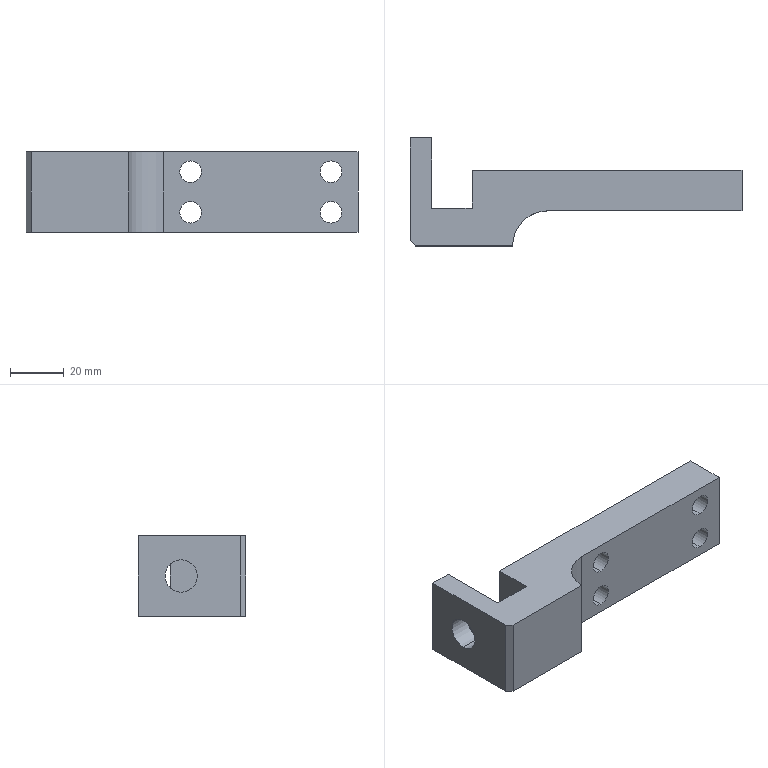Part | SolidWorks | features BaseBody 1 | 1 solid | 23 faces | box 123 x 40 x 30 mm | volume 63857 mm3 | plane 12 | cylinder 11 | commonest cylinder face diameters 8 x8 12 x2 26 x1
STEP:
#1=CARTESIAN_POINT('',(340.,-80.,88.121));
#2=VERTEX_POINT('',#1);
#3=CARTESIAN_POINT('',(340.,-80.,96.121));
#4=VERTEX_POINT('',#3);
#5=CARTESIAN_POINT('',(340.,-80.,92.121));
#6=DIRECTION('',(0.,1.,0.));
#7=DIRECTION('',(0.,0.,-1.));
#8=AXIS2_PLACEMENT_3D('',#5,#6,#7);
#9=CIRCLE('',#8,4.);
#10=EDGE_CURVE('',#2,#4,#9,.T.);
#11=ORIENTED_EDGE('',*,*,#10,.T.);
#12=CARTESIAN_POINT('',(340.,-95.,96.121));
#13=VERTEX_POINT('',#12);
#14=CARTESIAN_POINT('',(340.,-95.,96.121));
#15=DIRECTION('',(0.,-1.,0.));
#16=VECTOR('',#15,1000.);
#17=LINE('',#14,#16);
#18=EDGE_CURVE('',#4,#13,#17,.T.);
#19=ORIENTED_EDGE('',*,*,#18,.T.);
#20=CARTESIAN_POINT('',(340.,-95.,88.121));
#21=VERTEX_POINT('',#20);
#22=CARTESIAN_POINT('',(340.,-95.,92.121));
#23=DIRECTION('',(0.,1.,0.));
#24=DIRECTION('',(0.,0.,-1.));
#25=AXIS2_PLACEMENT_3D('',#22,#23,#24);
#26=CIRCLE('',#25,4.);
#27=EDGE_CURVE('',#21,#13,#26,.T.);
#28=ORIENTED_EDGE('',*,*,#27,.F.);
#29=CARTESIAN_POINT('',(340.,-95.,88.121));
#30=DIRECTION('',(0.,-1.,0.));
#31=VECTOR('',#30,1000.);
#32=LINE('',#29,#31);
#33=EDGE_CURVE('',#2,#21,#32,.T.);
#34=ORIENTED_EDGE('',*,*,#33,.F.);
#35=EDGE_LOOP('',(#11,#19,#28,#34));
#36=FACE_OUTER_BOUND('',#35,.T.);
#37=CARTESIAN_POINT('',(340.,-95.,92.121));
#38=DIRECTION('',(0.,-1.,0.));
#39=DIRECTION('',(0.,0.,-1.));
#40=AXIS2_PLACEMENT_3D('',#37,#38,#39);
#41=CYLINDRICAL_SURFACE('',#40,4.);
#42=ADVANCED_FACE('',(#36),#41,.F.);
#43=CARTESIAN_POINT('',(340.,-80.,103.121));
#44=VERTEX_POINT('',#43);
#45=CARTESIAN_POINT('',(340.,-80.,111.121));
#46=VERTEX_POINT('',#45);
#47=CARTESIAN_POINT('',(340.,-80.,107.121));
#48=DIRECTION('',(0.,1.,0.));
#49=DIRECTION('',(0.,0.,-1.));
#50=AXIS2_PLACEMENT_3D('',#47,#48,#49);
#51=CIRCLE('',#50,4.);
#52=EDGE_CURVE('',#44,#46,#51,.T.);
#53=ORIENTED_EDGE('',*,*,#52,.T.);
#54=CARTESIAN_POINT('',(340.,-95.,111.121));
#55=VERTEX_POINT('',#54);
#56=CARTESIAN_POINT('',(340.,-95.,111.121));
#57=DIRECTION('',(0.,-1.,0.));
#58=VECTOR('',#57,1000.);
#59=LINE('',#56,#58);
#60=EDGE_CURVE('',#46,#55,#59,.T.);
#61=ORIENTED_EDGE('',*,*,#60,.T.);
#62=CARTESIAN_POINT('',(340.,-95.,103.121));
#63=VERTEX_POINT('',#62);
#64=CARTESIAN_POINT('',(340.,-95.,107.121));
#65=DIRECTION('',(0.,1.,0.));
#66=DIRECTION('',(0.,0.,-1.));
#67=AXIS2_PLACEMENT_3D('',#64,#65,#66);
#68=CIRCLE('',#67,4.);
#69=EDGE_CURVE('',#63,#55,#68,.T.);
#70=ORIENTED_EDGE('',*,*,#69,.F.);
#71=CARTESIAN_POINT('',(340.,-95.,103.121));
#72=DIRECTION('',(0.,-1.,0.));
#73=VECTOR('',#72,1000.);
#74=LINE('',#71,#73);
#75=EDGE_CURVE('',#44,#63,#74,.T.);
#76=ORIENTED_EDGE('',*,*,#75,.F.);
#77=EDGE_LOOP('',(#53,#61,#70,#76));
#78=FACE_OUTER_BOUND('',#77,.T.);
#79=CARTESIAN_POINT('',(340.,-95.,107.121));
#80=DIRECTION('',(0.,-1.,0.));
#81=DIRECTION('',(0.,0.,-1.));
#82=AXIS2_PLACEMENT_3D('',#79,#80,#81);
#83=CYLINDRICAL_SURFACE('',#82,4.);
#84=ADVANCED_FACE('',(#78),#83,.F.);
#85=CARTESIAN_POINT('',(288.,-80.,103.121));
#86=VERTEX_POINT('',#85);
#87=CARTESIAN_POINT('',(288.,-80.,111.121));
#88=VERTEX_POINT('',#87);
#89=CARTESIAN_POINT('',(288.,-80.,107.121));
#90=DIRECTION('',(0.,1.,0.));
#91=DIRECTION('',(0.,0.,-1.));
#92=AXIS2_PLACEMENT_3D('',#89,#90,#91);
#93=CIRCLE('',#92,4.);
#94=EDGE_CURVE('',#86,#88,#93,.T.);
#95=ORIENTED_EDGE('',*,*,#94,.T.);
#96=CARTESIAN_POINT('',(288.,-95.,111.121));
#97=VERTEX_POINT('',#96);
#98=CARTESIAN_POINT('',(288.,-95.,111.121));
#99=DIRECTION('',(0.,-1.,0.));
#100=VECTOR('',#99,1000.);
#101=LINE('',#98,#100);
#102=EDGE_CURVE('',#88,#97,#101,.T.);
#103=ORIENTED_EDGE('',*,*,#102,.T.);
#104=CARTESIAN_POINT('',(288.,-95.,103.121));
#105=VERTEX_POINT('',#104);
#106=CARTESIAN_POINT('',(288.,-95.,107.121));
#107=DIRECTION('',(0.,1.,0.));
#108=DIRECTION('',(0.,0.,-1.));
#109=AXIS2_PLACEMENT_3D('',#106,#107,#108);
#110=CIRCLE('',#109,4.);
#111=EDGE_CURVE('',#105,#97,#110,.T.);
#112=ORIENTED_EDGE('',*,*,#111,.F.);
#113=CARTESIAN_POINT('',(288.,-95.,103.121));
#114=DIRECTION('',(0.,-1.,0.));
#115=VECTOR('',#114,1000.);
#116=LINE('',#113,#115);
#117=EDGE_CURVE('',#86,#105,#116,.T.);
#118=ORIENTED_EDGE('',*,*,#117,.F.);
#119=EDGE_LOOP('',(#95,#103,#112,#118));
#120=FACE_OUTER_BOUND('',#119,.T.);
#121=CARTESIAN_POINT('',(288.,-95.,107.121));
#122=DIRECTION('',(0.,-1.,0.));
#123=DIRECTION('',(0.,0.,-1.));
#124=AXIS2_PLACEMENT_3D('',#121,#122,#123);
#125=CYLINDRICAL_SURFACE('',#124,4.);
#126=ADVANCED_FACE('',(#120),#125,.F.);
#127=CARTESIAN_POINT('',(288.,-80.,88.121));
#128=VERTEX_POINT('',#127);
#129=CARTESIAN_POINT('',(288.,-80.,96.121));
#130=VERTEX_POINT('',#129);
#131=CARTESIAN_POINT('',(288.,-80.,92.121));
#132=DIRECTION('',(0.,1.,0.));
#133=DIRECTION('',(0.,0.,-1.));
#134=AXIS2_PLACEMENT_3D('',#131,#132,#133);
#135=CIRCLE('',#134,4.);
#136=EDGE_CURVE('',#128,#130,#135,.T.);
#137=ORIENTED_EDGE('',*,*,#136,.T.);
#138=CARTESIAN_POINT('',(288.,-95.,96.121));
#139=VERTEX_POINT('',#138);
#140=CARTESIAN_POINT('',(288.,-95.,96.121));
#141=DIRECTION('',(0.,-1.,0.));
#142=VECTOR('',#141,1000.);
#143=LINE('',#140,#142);
#144=EDGE_CURVE('',#130,#139,#143,.T.);
#145=ORIENTED_EDGE('',*,*,#144,.T.);
#146=CARTESIAN_POINT('',(288.,-95.,88.121));
#147=VERTEX_POINT('',#146);
#148=CARTESIAN_POINT('',(288.,-95.,92.121));
#149=DIRECTION('',(0.,1.,0.));
#150=DIRECTION('',(0.,0.,-1.));
#151=AXIS2_PLACEMENT_3D('',#148,#149,#150);
#152=CIRCLE('',#151,4.);
#153=EDGE_CURVE('',#147,#139,#152,.T.);
#154=ORIENTED_EDGE('',*,*,#153,.F.);
#155=CARTESIAN_POINT('',(288.,-95.,88.121));
#156=DIRECTION('',(0.,-1.,0.));
#157=VECTOR('',#156,1000.);
#158=LINE('',#155,#157);
#159=EDGE_CURVE('',#128,#147,#158,.T.);
#160=ORIENTED_EDGE('',*,*,#159,.F.);
#161=EDGE_LOOP('',(#137,#145,#154,#160));
#162=FACE_OUTER_BOUND('',#161,.T.);
#163=CARTESIAN_POINT('',(288.,-95.,92.121));
#164=DIRECTION('',(0.,-1.,0.));
#165=DIRECTION('',(0.,0.,-1.));
#166=AXIS2_PLACEMENT_3D('',#163,#164,#165);
#167=CYLINDRICAL_SURFACE('',#166,4.);
#168=ADVANCED_FACE('',(#162),#167,.F.);
#169=CARTESIAN_POINT('',(235.,-84.,105.621));
#170=VERTEX_POINT('',#169);
#171=CARTESIAN_POINT('',(235.,-84.,93.621));
#172=VERTEX_POINT('',#171);
#173=CARTESIAN_POINT('',(235.,-84.,99.621));
#174=DIRECTION('',(1.,0.,0.));
#175=DIRECTION('',(0.,0.,1.));
#176=AXIS2_PLACEMENT_3D('',#173,#174,#175);
#177=CIRCLE('',#176,6.);
#178=EDGE_CURVE('',#170,#172,#177,.T.);
#179=ORIENTED_EDGE('',*,*,#178,.T.);
#180=CARTESIAN_POINT('',(227.,-84.,93.621));
#181=VERTEX_POINT('',#180);
#182=CARTESIAN_POINT('',(251.971,-84.,93.621));
#183=DIRECTION('',(-1.,0.,0.));
#184=VECTOR('',#183,1000.);
#185=LINE('',#182,#184);
#186=EDGE_CURVE('',#172,#181,#185,.T.);
#187=ORIENTED_EDGE('',*,*,#186,.T.);
#188=CARTESIAN_POINT('',(227.,-84.,105.621));
#189=VERTEX_POINT('',#188);
#190=CARTESIAN_POINT('',(227.,-84.,99.621));
#191=DIRECTION('',(-1.,0.,0.));
#192=DIRECTION('',(0.,0.,1.));
#193=AXIS2_PLACEMENT_3D('',#190,#191,#192);
#194=CIRCLE('',#193,6.);
#195=EDGE_CURVE('',#181,#189,#194,.T.);
#196=ORIENTED_EDGE('',*,*,#195,.T.);
#197=CARTESIAN_POINT('',(251.971,-84.,105.621));
#198=DIRECTION('',(-1.,0.,0.));
#199=VECTOR('',#198,1000.);
#200=LINE('',#197,#199);
#201=EDGE_CURVE('',#170,#189,#200,.T.);
#202=ORIENTED_EDGE('',*,*,#201,.F.);
#203=EDGE_LOOP('',(#179,#187,#196,#202));
#204=FACE_OUTER_BOUND('',#203,.T.);
#205=CARTESIAN_POINT('',(251.971,-84.,99.621));
#206=DIRECTION('',(-1.,0.,0.));
#207=DIRECTION('',(0.,0.,1.));
#208=AXIS2_PLACEMENT_3D('',#205,#206,#207);
#209=CYLINDRICAL_SURFACE('',#208,6.);
#210=ADVANCED_FACE('',(#204),#209,.F.);
#211=CARTESIAN_POINT('',(350.,-80.,84.621));
#212=VERTEX_POINT('',#211);
#213=CARTESIAN_POINT('',(350.,-80.,114.621));
#214=VERTEX_POINT('',#213);
#215=CARTESIAN_POINT('',(350.,-80.,84.621));
#216=DIRECTION('',(0.,0.,1.));
#217=VECTOR('',#216,1000.);
#218=LINE('',#215,#217);
#219=EDGE_CURVE('',#212,#214,#218,.T.);
#220=ORIENTED_EDGE('',*,*,#219,.F.);
#221=CARTESIAN_POINT('',(250.,-80.,84.621));
#222=VERTEX_POINT('',#221);
#223=CARTESIAN_POINT('',(350.,-80.,84.621));
#224=DIRECTION('',(1.,0.,0.));
#225=VECTOR('',#224,1000.);
#226=LINE('',#223,#225);
#227=EDGE_CURVE('',#222,#212,#226,.T.);
#228=ORIENTED_EDGE('',*,*,#227,.F.);
#229=CARTESIAN_POINT('',(250.,-80.,114.621));
#230=VERTEX_POINT('',#229);
#231=CARTESIAN_POINT('',(250.,-80.,84.621));
#232=DIRECTION('',(0.,0.,-1.));
#233=VECTOR('',#232,1000.);
#234=LINE('',#231,#233);
#235=EDGE_CURVE('',#230,#222,#234,.T.);
#236=ORIENTED_EDGE('',*,*,#235,.F.);
#237=CARTESIAN_POINT('',(350.,-80.,114.621));
#238=DIRECTION('',(-1.,0.,0.));
#239=VECTOR('',#238,1000.);
#240=LINE('',#237,#239);
#241=EDGE_CURVE('',#214,#230,#240,.T.);
#242=ORIENTED_EDGE('',*,*,#241,.F.);
#243=EDGE_LOOP('',(#220,#228,#236,#242));
#244=FACE_OUTER_BOUND('',#243,.T.);
#245=ORIENTED_EDGE('',*,*,#10,.F.);
#246=CARTESIAN_POINT('',(340.,-80.,92.121));
#247=DIRECTION('',(0.,1.,0.));
#248=DIRECTION('',(0.,0.,-1.));
#249=AXIS2_PLACEMENT_3D('',#246,#247,#248);
#250=CIRCLE('',#249,4.);
#251=EDGE_CURVE('',#4,#2,#250,.T.);
#252=ORIENTED_EDGE('',*,*,#251,.F.);
#253=EDGE_LOOP('',(#245,#252));
#254=FACE_BOUND('',#253,.T.);
#255=ORIENTED_EDGE('',*,*,#52,.F.);
#256=CARTESIAN_POINT('',(340.,-80.,107.121));
#257=DIRECTION('',(0.,1.,0.));
#258=DIRECTION('',(0.,0.,-1.));
#259=AXIS2_PLACEMENT_3D('',#256,#257,#258);
#260=CIRCLE('',#259,4.);
#261=EDGE_CURVE('',#46,#44,#260,.T.);
#262=ORIENTED_EDGE('',*,*,#261,.F.);
#263=EDGE_LOOP('',(#255,#262));
#264=FACE_BOUND('',#263,.T.);
#265=ORIENTED_EDGE('',*,*,#94,.F.);
#266=CARTESIAN_POINT('',(288.,-80.,107.121));
#267=DIRECTION('',(0.,1.,0.));
#268=DIRECTION('',(0.,0.,-1.));
#269=AXIS2_PLACEMENT_3D('',#266,#267,#268);
#270=CIRCLE('',#269,4.);
#271=EDGE_CURVE('',#88,#86,#270,.T.);
#272=ORIENTED_EDGE('',*,*,#271,.F.);
#273=EDGE_LOOP('',(#265,#272));
#274=FACE_BOUND('',#273,.T.);
#275=ORIENTED_EDGE('',*,*,#136,.F.);
#276=CARTESIAN_POINT('',(288.,-80.,92.121));
#277=DIRECTION('',(0.,1.,0.));
#278=DIRECTION('',(0.,0.,-1.));
#279=AXIS2_PLACEMENT_3D('',#276,#277,#278);
#280=CIRCLE('',#279,4.);
#281=EDGE_CURVE('',#130,#128,#280,.T.);
#282=ORIENTED_EDGE('',*,*,#281,.F.);
#283=EDGE_LOOP('',(#275,#282));
#284=FACE_BOUND('',#283,.T.);
#285=CARTESIAN_POINT('',(350.,-80.,84.621));
#286=DIRECTION('',(0.,-1.,0.));
#287=DIRECTION('',(0.,0.,-1.));
#288=AXIS2_PLACEMENT_3D('',#285,#286,#287);
#289=PLANE('',#288);
#290=ADVANCED_FACE('',(#244,#254,#264,#274,#284),#289,.F.);
#291=CARTESIAN_POINT('',(229.,-108.,114.621));
#292=VERTEX_POINT('',#291);
#293=CARTESIAN_POINT('',(227.,-106.,114.621));
#294=VERTEX_POINT('',#293);
#295=CARTESIAN_POINT('',(229.,-108.,114.621));
#296=DIRECTION('',(-0.7071,0.7071,0.));
#297=VECTOR('',#296,1000.);
#298=LINE('',#295,#297);
#299=EDGE_CURVE('',#292,#294,#298,.T.);
#300=ORIENTED_EDGE('',*,*,#299,.F.);
#301=CARTESIAN_POINT('',(265.,-108.,114.621));
#302=VERTEX_POINT('',#301);
#303=CARTESIAN_POINT('',(251.867,-108.,114.621));
#304=DIRECTION('',(-1.,0.,0.));
#305=VECTOR('',#304,1000.);
#306=LINE('',#303,#305);
#307=EDGE_CURVE('',#302,#292,#306,.T.);
#308=ORIENTED_EDGE('',*,*,#307,.F.);
#309=CARTESIAN_POINT('',(278.,-95.,114.621));
#310=VERTEX_POINT('',#309);
#311=CARTESIAN_POINT('',(278.,-108.,114.621));
#312=DIRECTION('',(0.,0.,1.));
#313=DIRECTION('',(-1.,0.,0.));
#314=AXIS2_PLACEMENT_3D('',#311,#312,#313);
#315=CIRCLE('',#314,13.);
#316=EDGE_CURVE('',#310,#302,#315,.T.);
#317=ORIENTED_EDGE('',*,*,#316,.F.);
#318=CARTESIAN_POINT('',(350.,-95.,114.621));
#319=VERTEX_POINT('',#318);
#320=CARTESIAN_POINT('',(251.867,-95.,114.621));
#321=DIRECTION('',(-1.,0.,0.));
#322=VECTOR('',#321,1000.);
#323=LINE('',#320,#322);
#324=EDGE_CURVE('',#319,#310,#323,.T.);
#325=ORIENTED_EDGE('',*,*,#324,.F.);
#326=CARTESIAN_POINT('',(350.,-82.6,114.621));
#327=DIRECTION('',(0.,-1.,0.));
#328=VECTOR('',#327,1000.);
#329=LINE('',#326,#328);
#330=EDGE_CURVE('',#214,#319,#329,.T.);
#331=ORIENTED_EDGE('',*,*,#330,.F.);
#332=ORIENTED_EDGE('',*,*,#241,.T.);
#333=CARTESIAN_POINT('',(250.,-94.,114.621));
#334=VERTEX_POINT('',#333);
#335=CARTESIAN_POINT('',(250.,-82.6,114.621));
#336=DIRECTION('',(0.,1.,0.));
#337=VECTOR('',#336,1000.);
#338=LINE('',#335,#337);
#339=EDGE_CURVE('',#334,#230,#338,.T.);
#340=ORIENTED_EDGE('',*,*,#339,.F.);
#341=CARTESIAN_POINT('',(235.,-94.,114.621));
#342=VERTEX_POINT('',#341);
#343=CARTESIAN_POINT('',(251.867,-94.,114.621));
#344=DIRECTION('',(1.,0.,0.));
#345=VECTOR('',#344,1000.);
#346=LINE('',#343,#345);
#347=EDGE_CURVE('',#342,#334,#346,.T.);
#348=ORIENTED_EDGE('',*,*,#347,.F.);
#349=CARTESIAN_POINT('',(235.,-68.,114.621));
#350=VERTEX_POINT('',#349);
#351=CARTESIAN_POINT('',(235.,-82.6,114.621));
#352=DIRECTION('',(0.,-1.,0.));
#353=VECTOR('',#352,1000.);
#354=LINE('',#351,#353);
#355=EDGE_CURVE('',#350,#342,#354,.T.);
#356=ORIENTED_EDGE('',*,*,#355,.F.);
#357=CARTESIAN_POINT('',(227.,-68.,114.621));
#358=VERTEX_POINT('',#357);
#359=CARTESIAN_POINT('',(251.867,-68.,114.621));
#360=DIRECTION('',(1.,0.,0.));
#361=VECTOR('',#360,1000.);
#362=LINE('',#359,#361);
#363=EDGE_CURVE('',#358,#350,#362,.T.);
#364=ORIENTED_EDGE('',*,*,#363,.F.);
#365=CARTESIAN_POINT('',(227.,-82.6,114.621));
#366=DIRECTION('',(0.,1.,0.));
#367=VECTOR('',#366,1000.);
#368=LINE('',#365,#367);
#369=EDGE_CURVE('',#294,#358,#368,.T.);
#370=ORIENTED_EDGE('',*,*,#369,.F.);
#371=EDGE_LOOP('',(#300,#308,#317,#325,#331,#332,#340,#348,#356,#364,#370));
#372=FACE_OUTER_BOUND('',#371,.T.);
#373=CARTESIAN_POINT('',(251.867,-82.6,114.621));
#374=DIRECTION('',(0.,0.,-1.));
#375=DIRECTION('',(-1.,0.,0.));
#376=AXIS2_PLACEMENT_3D('',#373,#374,#375);
#377=PLANE('',#376);
#378=ADVANCED_FACE('',(#372),#377,.F.);
#379=CARTESIAN_POINT('',(350.,-95.,84.621));
#380=VERTEX_POINT('',#379);
#381=CARTESIAN_POINT('',(350.,-95.,84.621));
#382=DIRECTION('',(0.,0.,1.));
#383=VECTOR('',#382,1000.);
#384=LINE('',#381,#383);
#385=EDGE_CURVE('',#380,#319,#384,.T.);
#386=ORIENTED_EDGE('',*,*,#385,.F.);
#387=CARTESIAN_POINT('',(350.,-80.,84.621));
#388=DIRECTION('',(0.,-1.,0.));
#389=VECTOR('',#388,1000.);
#390=LINE('',#387,#389);
#391=EDGE_CURVE('',#212,#380,#390,.T.);
#392=ORIENTED_EDGE('',*,*,#391,.F.);
#393=ORIENTED_EDGE('',*,*,#219,.T.);
#394=ORIENTED_EDGE('',*,*,#330,.T.);
#395=EDGE_LOOP('',(#386,#392,#393,#394));
#396=FACE_OUTER_BOUND('',#395,.T.);
#397=CARTESIAN_POINT('',(350.,-80.,84.621));
#398=DIRECTION('',(-1.,0.,0.));
#399=DIRECTION('',(0.,0.,1.));
#400=AXIS2_PLACEMENT_3D('',#397,#398,#399);
#401=PLANE('',#400);
#402=ADVANCED_FACE('',(#396),#401,.F.);
#403=CARTESIAN_POINT('',(278.,-95.,84.621));
#404=VERTEX_POINT('',#403);
#405=CARTESIAN_POINT('',(251.867,-95.,84.621));
#406=DIRECTION('',(-1.,0.,0.));
#407=VECTOR('',#406,1000.);
#408=LINE('',#405,#407);
#409=EDGE_CURVE('',#380,#404,#408,.T.);
#410=ORIENTED_EDGE('',*,*,#409,.T.);
#411=CARTESIAN_POINT('',(265.,-108.,84.621));
#412=VERTEX_POINT('',#411);
#413=CARTESIAN_POINT('',(278.,-108.,84.621));
#414=DIRECTION('',(0.,0.,1.));
#415=DIRECTION('',(-1.,0.,0.));
#416=AXIS2_PLACEMENT_3D('',#413,#414,#415);
#417=CIRCLE('',#416,13.);
#418=EDGE_CURVE('',#404,#412,#417,.T.);
#419=ORIENTED_EDGE('',*,*,#418,.T.);
#420=CARTESIAN_POINT('',(229.,-108.,84.621));
#421=VERTEX_POINT('',#420);
#422=CARTESIAN_POINT('',(251.867,-108.,84.621));
#423=DIRECTION('',(-1.,0.,0.));
#424=VECTOR('',#423,1000.);
#425=LINE('',#422,#424);
#426=EDGE_CURVE('',#412,#421,#425,.T.);
#427=ORIENTED_EDGE('',*,*,#426,.T.);
#428=CARTESIAN_POINT('',(227.,-106.,84.621));
#429=VERTEX_POINT('',#428);
#430=CARTESIAN_POINT('',(229.,-108.,84.621));
#431=DIRECTION('',(-0.7071,0.7071,0.));
#432=VECTOR('',#431,1000.);
#433=LINE('',#430,#432);
#434=EDGE_CURVE('',#421,#429,#433,.T.);
#435=ORIENTED_EDGE('',*,*,#434,.T.);
#436=CARTESIAN_POINT('',(227.,-68.,84.621));
#437=VERTEX_POINT('',#436);
#438=CARTESIAN_POINT('',(227.,-82.6,84.621));
#439=DIRECTION('',(0.,1.,0.));
#440=VECTOR('',#439,1000.);
#441=LINE('',#438,#440);
#442=EDGE_CURVE('',#429,#437,#441,.T.);
#443=ORIENTED_EDGE('',*,*,#442,.T.);
#444=CARTESIAN_POINT('',(235.,-68.,84.621));
#445=VERTEX_POINT('',#444);
#446=CARTESIAN_POINT('',(251.867,-68.,84.621));
#447=DIRECTION('',(1.,0.,0.));
#448=VECTOR('',#447,1000.);
#449=LINE('',#446,#448);
#450=EDGE_CURVE('',#437,#445,#449,.T.);
#451=ORIENTED_EDGE('',*,*,#450,.T.);
#452=CARTESIAN_POINT('',(235.,-94.,84.621));
#453=VERTEX_POINT('',#452);
#454=CARTESIAN_POINT('',(235.,-82.6,84.621));
#455=DIRECTION('',(0.,-1.,0.));
#456=VECTOR('',#455,1000.);
#457=LINE('',#454,#456);
#458=EDGE_CURVE('',#445,#453,#457,.T.);
#459=ORIENTED_EDGE('',*,*,#458,.T.);
#460=CARTESIAN_POINT('',(250.,-94.,84.621));
#461=VERTEX_POINT('',#460);
#462=CARTESIAN_POINT('',(251.867,-94.,84.621));
#463=DIRECTION('',(1.,0.,0.));
#464=VECTOR('',#463,1000.);
#465=LINE('',#462,#464);
#466=EDGE_CURVE('',#453,#461,#465,.T.);
#467=ORIENTED_EDGE('',*,*,#466,.T.);
#468=CARTESIAN_POINT('',(250.,-82.6,84.621));
#469=DIRECTION('',(0.,1.,0.));
#470=VECTOR('',#469,1000.);
#471=LINE('',#468,#470);
#472=EDGE_CURVE('',#461,#222,#471,.T.);
#473=ORIENTED_EDGE('',*,*,#472,.T.);
#474=ORIENTED_EDGE('',*,*,#227,.T.);
#475=ORIENTED_EDGE('',*,*,#391,.T.);
#476=EDGE_LOOP('',(#410,#419,#427,#435,#443,#451,#459,#467,#473,#474,#475));
#477=FACE_OUTER_BOUND('',#476,.T.);
#478=CARTESIAN_POINT('',(251.867,-82.6,84.621));
#479=DIRECTION('',(0.,0.,-1.));
#480=DIRECTION('',(-1.,0.,0.));
#481=AXIS2_PLACEMENT_3D('',#478,#479,#480);
#482=PLANE('',#481);
#483=ADVANCED_FACE('',(#477),#482,.T.);
#484=ORIENTED_EDGE('',*,*,#235,.T.);
#485=ORIENTED_EDGE('',*,*,#472,.F.);
#486=CARTESIAN_POINT('',(250.,-94.,84.621));
#487=DIRECTION('',(0.,0.,-1.));
#488=VECTOR('',#487,1000.);
#489=LINE('',#486,#488);
#490=EDGE_CURVE('',#334,#461,#489,.T.);
#491=ORIENTED_EDGE('',*,*,#490,.F.);
#492=ORIENTED_EDGE('',*,*,#339,.T.);
#493=EDGE_LOOP('',(#484,#485,#491,#492));
#494=FACE_OUTER_BOUND('',#493,.T.);
#495=CARTESIAN_POINT('',(250.,-80.,84.621));
#496=DIRECTION('',(1.,0.,0.));
#497=DIRECTION('',(0.,0.,-1.));
#498=AXIS2_PLACEMENT_3D('',#495,#496,#497);
#499=PLANE('',#498);
#500=ADVANCED_FACE('',(#494),#499,.F.);
#501=ORIENTED_EDGE('',*,*,#18,.F.);
#502=ORIENTED_EDGE('',*,*,#251,.T.);
#503=ORIENTED_EDGE('',*,*,#33,.T.);
#504=CARTESIAN_POINT('',(340.,-95.,92.121));
#505=DIRECTION('',(0.,1.,0.));
#506=DIRECTION('',(0.,0.,-1.));
#507=AXIS2_PLACEMENT_3D('',#504,#505,#506);
#508=CIRCLE('',#507,4.);
#509=EDGE_CURVE('',#13,#21,#508,.T.);
#510=ORIENTED_EDGE('',*,*,#509,.F.);
#511=EDGE_LOOP('',(#501,#502,#503,#510));
#512=FACE_OUTER_BOUND('',#511,.T.);
#513=CARTESIAN_POINT('',(340.,-95.,92.121));
#514=DIRECTION('',(0.,-1.,0.));
#515=DIRECTION('',(0.,0.,-1.));
#516=AXIS2_PLACEMENT_3D('',#513,#514,#515);
#517=CYLINDRICAL_SURFACE('',#516,4.);
#518=ADVANCED_FACE('',(#512),#517,.F.);
#519=ORIENTED_EDGE('',*,*,#60,.F.);
#520=ORIENTED_EDGE('',*,*,#261,.T.);
#521=ORIENTED_EDGE('',*,*,#75,.T.);
#522=CARTESIAN_POINT('',(340.,-95.,107.121));
#523=DIRECTION('',(0.,1.,0.));
#524=DIRECTION('',(0.,0.,-1.));
#525=AXIS2_PLACEMENT_3D('',#522,#523,#524);
#526=CIRCLE('',#525,4.);
#527=EDGE_CURVE('',#55,#63,#526,.T.);
#528=ORIENTED_EDGE('',*,*,#527,.F.);
#529=EDGE_LOOP('',(#519,#520,#521,#528));
#530=FACE_OUTER_BOUND('',#529,.T.);
#531=CARTESIAN_POINT('',(340.,-95.,107.121));
#532=DIRECTION('',(0.,-1.,0.));
#533=DIRECTION('',(0.,0.,-1.));
#534=AXIS2_PLACEMENT_3D('',#531,#532,#533);
#535=CYLINDRICAL_SURFACE('',#534,4.);
#536=ADVANCED_FACE('',(#530),#535,.F.);
#537=ORIENTED_EDGE('',*,*,#102,.F.);
#538=ORIENTED_EDGE('',*,*,#271,.T.);
#539=ORIENTED_EDGE('',*,*,#117,.T.);
#540=CARTESIAN_POINT('',(288.,-95.,107.121));
#541=DIRECTION('',(0.,1.,0.));
#542=DIRECTION('',(0.,0.,-1.));
#543=AXIS2_PLACEMENT_3D('',#540,#541,#542);
#544=CIRCLE('',#543,4.);
#545=EDGE_CURVE('',#97,#105,#544,.T.);
#546=ORIENTED_EDGE('',*,*,#545,.F.);
#547=EDGE_LOOP('',(#537,#538,#539,#546));
#548=FACE_OUTER_BOUND('',#547,.T.);
#549=CARTESIAN_POINT('',(288.,-95.,107.121));
#550=DIRECTION('',(0.,-1.,0.));
#551=DIRECTION('',(0.,0.,-1.));
#552=AXIS2_PLACEMENT_3D('',#549,#550,#551);
#553=CYLINDRICAL_SURFACE('',#552,4.);
#554=ADVANCED_FACE('',(#548),#553,.F.);
#555=ORIENTED_EDGE('',*,*,#144,.F.);
#556=ORIENTED_EDGE('',*,*,#281,.T.);
#557=ORIENTED_EDGE('',*,*,#159,.T.);
#558=CARTESIAN_POINT('',(288.,-95.,92.121));
#559=DIRECTION('',(0.,1.,0.));
#560=DIRECTION('',(0.,0.,-1.));
#561=AXIS2_PLACEMENT_3D('',#558,#559,#560);
#562=CIRCLE('',#561,4.);
#563=EDGE_CURVE('',#139,#147,#562,.T.);
#564=ORIENTED_EDGE('',*,*,#563,.F.);
#565=EDGE_LOOP('',(#555,#556,#557,#564));
#566=FACE_OUTER_BOUND('',#565,.T.);
#567=CARTESIAN_POINT('',(288.,-95.,92.121));
#568=DIRECTION('',(0.,-1.,0.));
#569=DIRECTION('',(0.,0.,-1.));
#570=AXIS2_PLACEMENT_3D('',#567,#568,#569);
#571=CYLINDRICAL_SURFACE('',#570,4.);
#572=ADVANCED_FACE('',(#566),#571,.F.);
#573=CARTESIAN_POINT('',(227.,-106.,84.621));
#574=DIRECTION('',(0.,0.,-1.));
#575=VECTOR('',#574,1000.);
#576=LINE('',#573,#575);
#577=EDGE_CURVE('',#294,#429,#576,.T.);
#578=ORIENTED_EDGE('',*,*,#577,.F.);
#579=ORIENTED_EDGE('',*,*,#369,.T.);
#580=CARTESIAN_POINT('',(227.,-68.,84.621));
#581=DIRECTION('',(0.,0.,1.));
#582=VECTOR('',#581,1000.);
#583=LINE('',#580,#582);
#584=EDGE_CURVE('',#437,#358,#583,.T.);
#585=ORIENTED_EDGE('',*,*,#584,.F.);
#586=ORIENTED_EDGE('',*,*,#442,.F.);
#587=EDGE_LOOP('',(#578,#579,#585,#586));
#588=FACE_OUTER_BOUND('',#587,.T.);
#589=CARTESIAN_POINT('',(227.,-84.,99.621));
#590=DIRECTION('',(-1.,0.,0.));
#591=DIRECTION('',(0.,0.,1.));
#592=AXIS2_PLACEMENT_3D('',#589,#590,#591);
#593=CIRCLE('',#592,6.);
#594=EDGE_CURVE('',#189,#181,#593,.T.);
#595=ORIENTED_EDGE('',*,*,#594,.F.);
#596=ORIENTED_EDGE('',*,*,#195,.F.);
#597=EDGE_LOOP('',(#595,#596));
#598=FACE_BOUND('',#597,.T.);
#599=CARTESIAN_POINT('',(227.,-93.,84.621));
#600=DIRECTION('',(1.,0.,0.));
#601=DIRECTION('',(0.,0.,-1.));
#602=AXIS2_PLACEMENT_3D('',#599,#600,#601);
#603=PLANE('',#602);
#604=ADVANCED_FACE('',(#588,#598),#603,.F.);
#605=CARTESIAN_POINT('',(229.,-108.,84.621));
#606=DIRECTION('',(0.,0.,-1.));
#607=VECTOR('',#606,1000.);
#608=LINE('',#605,#607);
#609=EDGE_CURVE('',#292,#421,#608,.T.);
#610=ORIENTED_EDGE('',*,*,#609,.F.);
#611=ORIENTED_EDGE('',*,*,#299,.T.);
#612=ORIENTED_EDGE('',*,*,#577,.T.);
#613=ORIENTED_EDGE('',*,*,#434,.F.);
#614=EDGE_LOOP('',(#610,#611,#612,#613));
#615=FACE_OUTER_BOUND('',#614,.T.);
#616=CARTESIAN_POINT('',(227.,-106.,84.621));
#617=DIRECTION('',(0.7071,0.7071,0.));
#618=DIRECTION('',(-0.7071,0.7071,0.));
#619=AXIS2_PLACEMENT_3D('',#616,#617,#618);
#620=PLANE('',#619);
#621=ADVANCED_FACE('',(#615),#620,.F.);
#622=ORIENTED_EDGE('',*,*,#609,.T.);
#623=ORIENTED_EDGE('',*,*,#426,.F.);
#624=CARTESIAN_POINT('',(265.,-108.,84.621));
#625=DIRECTION('',(0.,0.,-1.));
#626=VECTOR('',#625,1000.);
#627=LINE('',#624,#626);
#628=EDGE_CURVE('',#302,#412,#627,.T.);
#629=ORIENTED_EDGE('',*,*,#628,.F.);
#630=ORIENTED_EDGE('',*,*,#307,.T.);
#631=EDGE_LOOP('',(#622,#623,#629,#630));
#632=FACE_OUTER_BOUND('',#631,.T.);
#633=CARTESIAN_POINT('',(265.,-108.,84.621));
#634=DIRECTION('',(0.,1.,0.));
#635=DIRECTION('',(0.,0.,1.));
#636=AXIS2_PLACEMENT_3D('',#633,#634,#635);
#637=PLANE('',#636);
#638=ADVANCED_FACE('',(#632),#637,.F.);
#639=CARTESIAN_POINT('',(278.,-95.,84.621));
#640=DIRECTION('',(0.,0.,-1.));
#641=VECTOR('',#640,1000.);
#642=LINE('',#639,#641);
#643=EDGE_CURVE('',#310,#404,#642,.T.);
#644=ORIENTED_EDGE('',*,*,#643,.F.);
#645=ORIENTED_EDGE('',*,*,#316,.T.);
#646=ORIENTED_EDGE('',*,*,#628,.T.);
#647=ORIENTED_EDGE('',*,*,#418,.F.);
#648=EDGE_LOOP('',(#644,#645,#646,#647));
#649=FACE_OUTER_BOUND('',#648,.T.);
#650=CARTESIAN_POINT('',(278.,-108.,84.621));
#651=DIRECTION('',(0.,0.,-1.));
#652=DIRECTION('',(-1.,0.,0.));
#653=AXIS2_PLACEMENT_3D('',#650,#651,#652);
#654=CYLINDRICAL_SURFACE('',#653,13.);
#655=ADVANCED_FACE('',(#649),#654,.F.);
#656=ORIENTED_EDGE('',*,*,#643,.T.);
#657=ORIENTED_EDGE('',*,*,#409,.F.);
#658=ORIENTED_EDGE('',*,*,#385,.T.);
#659=ORIENTED_EDGE('',*,*,#324,.T.);
#660=EDGE_LOOP('',(#656,#657,#658,#659));
#661=FACE_OUTER_BOUND('',#660,.T.);
#662=ORIENTED_EDGE('',*,*,#27,.T.);
#663=ORIENTED_EDGE('',*,*,#509,.T.);
#664=EDGE_LOOP('',(#662,#663));
#665=FACE_BOUND('',#664,.T.);
#666=ORIENTED_EDGE('',*,*,#69,.T.);
#667=ORIENTED_EDGE('',*,*,#527,.T.);
#668=EDGE_LOOP('',(#666,#667));
#669=FACE_BOUND('',#668,.T.);
#670=ORIENTED_EDGE('',*,*,#111,.T.);
#671=ORIENTED_EDGE('',*,*,#545,.T.);
#672=EDGE_LOOP('',(#670,#671));
#673=FACE_BOUND('',#672,.T.);
#674=ORIENTED_EDGE('',*,*,#153,.T.);
#675=ORIENTED_EDGE('',*,*,#563,.T.);
#676=EDGE_LOOP('',(#674,#675));
#677=FACE_BOUND('',#676,.T.);
#678=CARTESIAN_POINT('',(350.,-95.,84.621));
#679=DIRECTION('',(0.,1.,0.));
#680=DIRECTION('',(0.,0.,1.));
#681=AXIS2_PLACEMENT_3D('',#678,#679,#680);
#682=PLANE('',#681);
#683=ADVANCED_FACE('',(#661,#665,#669,#673,#677),#682,.F.);
#684=ORIENTED_EDGE('',*,*,#490,.T.);
#685=ORIENTED_EDGE('',*,*,#466,.F.);
#686=CARTESIAN_POINT('',(235.,-94.,84.621));
#687=DIRECTION('',(0.,0.,-1.));
#688=VECTOR('',#687,1000.);
#689=LINE('',#686,#688);
#690=EDGE_CURVE('',#342,#453,#689,.T.);
#691=ORIENTED_EDGE('',*,*,#690,.F.);
#692=ORIENTED_EDGE('',*,*,#347,.T.);
#693=EDGE_LOOP('',(#684,#685,#691,#692));
#694=FACE_OUTER_BOUND('',#693,.T.);
#695=CARTESIAN_POINT('',(250.,-94.,84.621));
#696=DIRECTION('',(0.,-1.,0.));
#697=DIRECTION('',(0.,0.,-1.));
#698=AXIS2_PLACEMENT_3D('',#695,#696,#697);
#699=PLANE('',#698);
#700=ADVANCED_FACE('',(#694),#699,.F.);
#701=ORIENTED_EDGE('',*,*,#690,.T.);
#702=ORIENTED_EDGE('',*,*,#458,.F.);
#703=CARTESIAN_POINT('',(235.,-68.,84.621));
#704=DIRECTION('',(0.,0.,-1.));
#705=VECTOR('',#704,1000.);
#706=LINE('',#703,#705);
#707=EDGE_CURVE('',#350,#445,#706,.T.);
#708=ORIENTED_EDGE('',*,*,#707,.F.);
#709=ORIENTED_EDGE('',*,*,#355,.T.);
#710=EDGE_LOOP('',(#701,#702,#708,#709));
#711=FACE_OUTER_BOUND('',#710,.T.);
#712=ORIENTED_EDGE('',*,*,#178,.F.);
#713=CARTESIAN_POINT('',(235.,-84.,99.621));
#714=DIRECTION('',(1.,0.,0.));
#715=DIRECTION('',(0.,0.,1.));
#716=AXIS2_PLACEMENT_3D('',#713,#714,#715);
#717=CIRCLE('',#716,6.);
#718=EDGE_CURVE('',#172,#170,#717,.T.);
#719=ORIENTED_EDGE('',*,*,#718,.F.);
#720=EDGE_LOOP('',(#712,#719));
#721=FACE_BOUND('',#720,.T.);
#722=CARTESIAN_POINT('',(235.,-94.,84.621));
#723=DIRECTION('',(-1.,0.,0.));
#724=DIRECTION('',(0.,0.,1.));
#725=AXIS2_PLACEMENT_3D('',#722,#723,#724);
#726=PLANE('',#725);
#727=ADVANCED_FACE('',(#711,#721),#726,.F.);
#728=ORIENTED_EDGE('',*,*,#707,.T.);
#729=ORIENTED_EDGE('',*,*,#450,.F.);
#730=ORIENTED_EDGE('',*,*,#584,.T.);
#731=ORIENTED_EDGE('',*,*,#363,.T.);
#732=EDGE_LOOP('',(#728,#729,#730,#731));
#733=FACE_OUTER_BOUND('',#732,.T.);
#734=CARTESIAN_POINT('',(227.,-68.,84.621));
#735=DIRECTION('',(0.,-1.,0.));
#736=DIRECTION('',(0.,0.,-1.));
#737=AXIS2_PLACEMENT_3D('',#734,#735,#736);
#738=PLANE('',#737);
#739=ADVANCED_FACE('',(#733),#738,.F.);
#740=ORIENTED_EDGE('',*,*,#186,.F.);
#741=ORIENTED_EDGE('',*,*,#718,.T.);
#742=ORIENTED_EDGE('',*,*,#201,.T.);
#743=ORIENTED_EDGE('',*,*,#594,.T.);
#744=EDGE_LOOP('',(#740,#741,#742,#743));
#745=FACE_OUTER_BOUND('',#744,.T.);
#746=CARTESIAN_POINT('',(251.971,-84.,99.621));
#747=DIRECTION('',(-1.,0.,0.));
#748=DIRECTION('',(0.,0.,1.));
#749=AXIS2_PLACEMENT_3D('',#746,#747,#748);
#750=CYLINDRICAL_SURFACE('',#749,6.);
#751=ADVANCED_FACE('',(#745),#750,.F.);
#752=CLOSED_SHELL('',(#42,#84,#126,#168,#210,#290,#378,#402,#483,#500,#518,#536,#554,#572,#604,#621,#638,#655,#683,#700,#727,#739,#751));
#753=MANIFOLD_SOLID_BREP('',#752);
#754=CARTESIAN_POINT('',(0.,0.,0.));
#755=DIRECTION('',(0.,0.,1.));
#756=DIRECTION('',(1.,0.,0.));
#757=AXIS2_PLACEMENT_3D('',#754,#755,#756);
#758=(LENGTH_UNIT()NAMED_UNIT(*)SI_UNIT(.MILLI.,.METRE.));
#759=UNCERTAINTY_MEASURE_WITH_UNIT(LENGTH_MEASURE(0.00001),#758,'','');
#760=(NAMED_UNIT(*)PLANE_ANGLE_UNIT()SI_UNIT($,.RADIAN.));
#761=(NAMED_UNIT(*)SI_UNIT($,.STERADIAN.)SOLID_ANGLE_UNIT());
#762=(GEOMETRIC_REPRESENTATION_CONTEXT(3)GLOBAL_UNCERTAINTY_ASSIGNED_CONTEXT((#759))GLOBAL_UNIT_ASSIGNED_CONTEXT((#758,#760,#761))REPRESENTATION_CONTEXT('',''));
#763=ADVANCED_BREP_SHAPE_REPRESENTATION('',(#753,#757),#762);